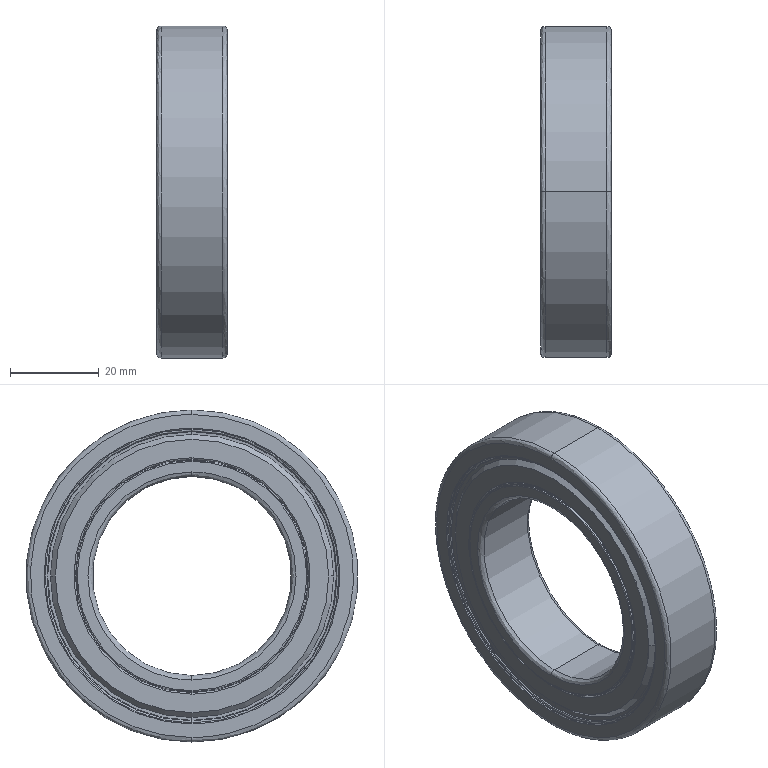Part | SolidWorks | features BaseBody 1 | 1 solid | 82 faces | box 16 x 75 x 75 mm | volume 36953 mm3 | spline 32 | cylinder 22 | cone 20 | plane 8 | commonest cylinder face diameters 53.6 x4 64.4 x4 45 x2 51.3 x2 52.2 x2 52.8 x2